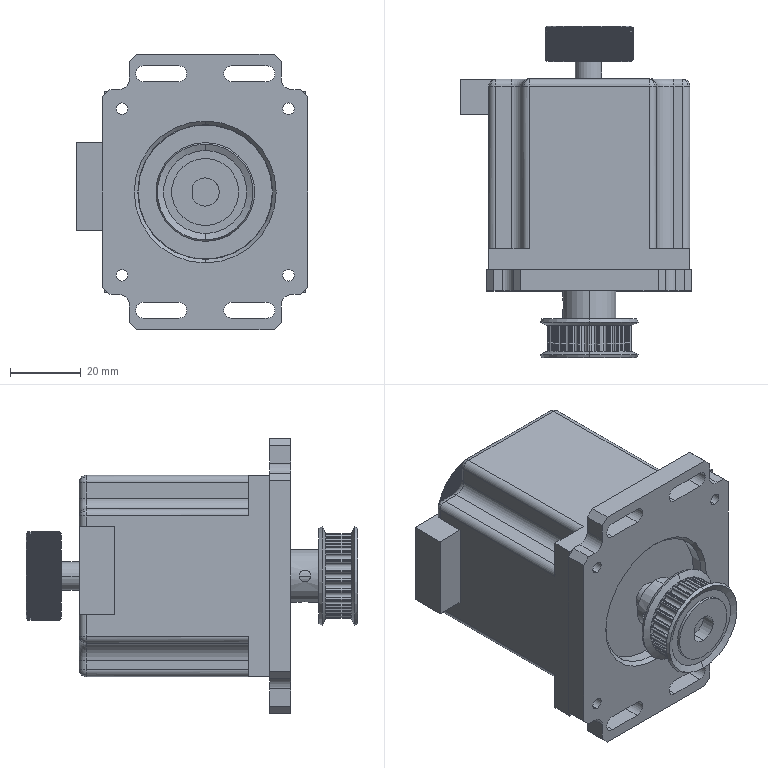Part | NX | features BREP 4 | 4 solids | 1582 faces | box 65.5 x 93.95 x 78 mm | volume 190120 mm3 | plane 914 | cylinder 625 | cone 23 | sphere 16 | torus 4 | commonest cylinder face diameters 25 x371 1.02 x62 3.04 x52 1.7 x36 24.07 x27 4 x21